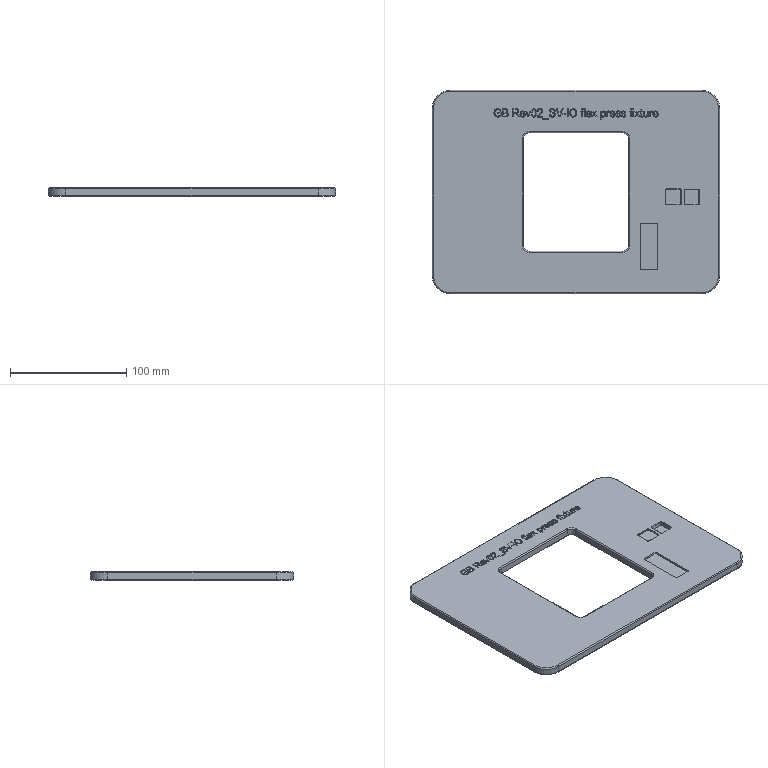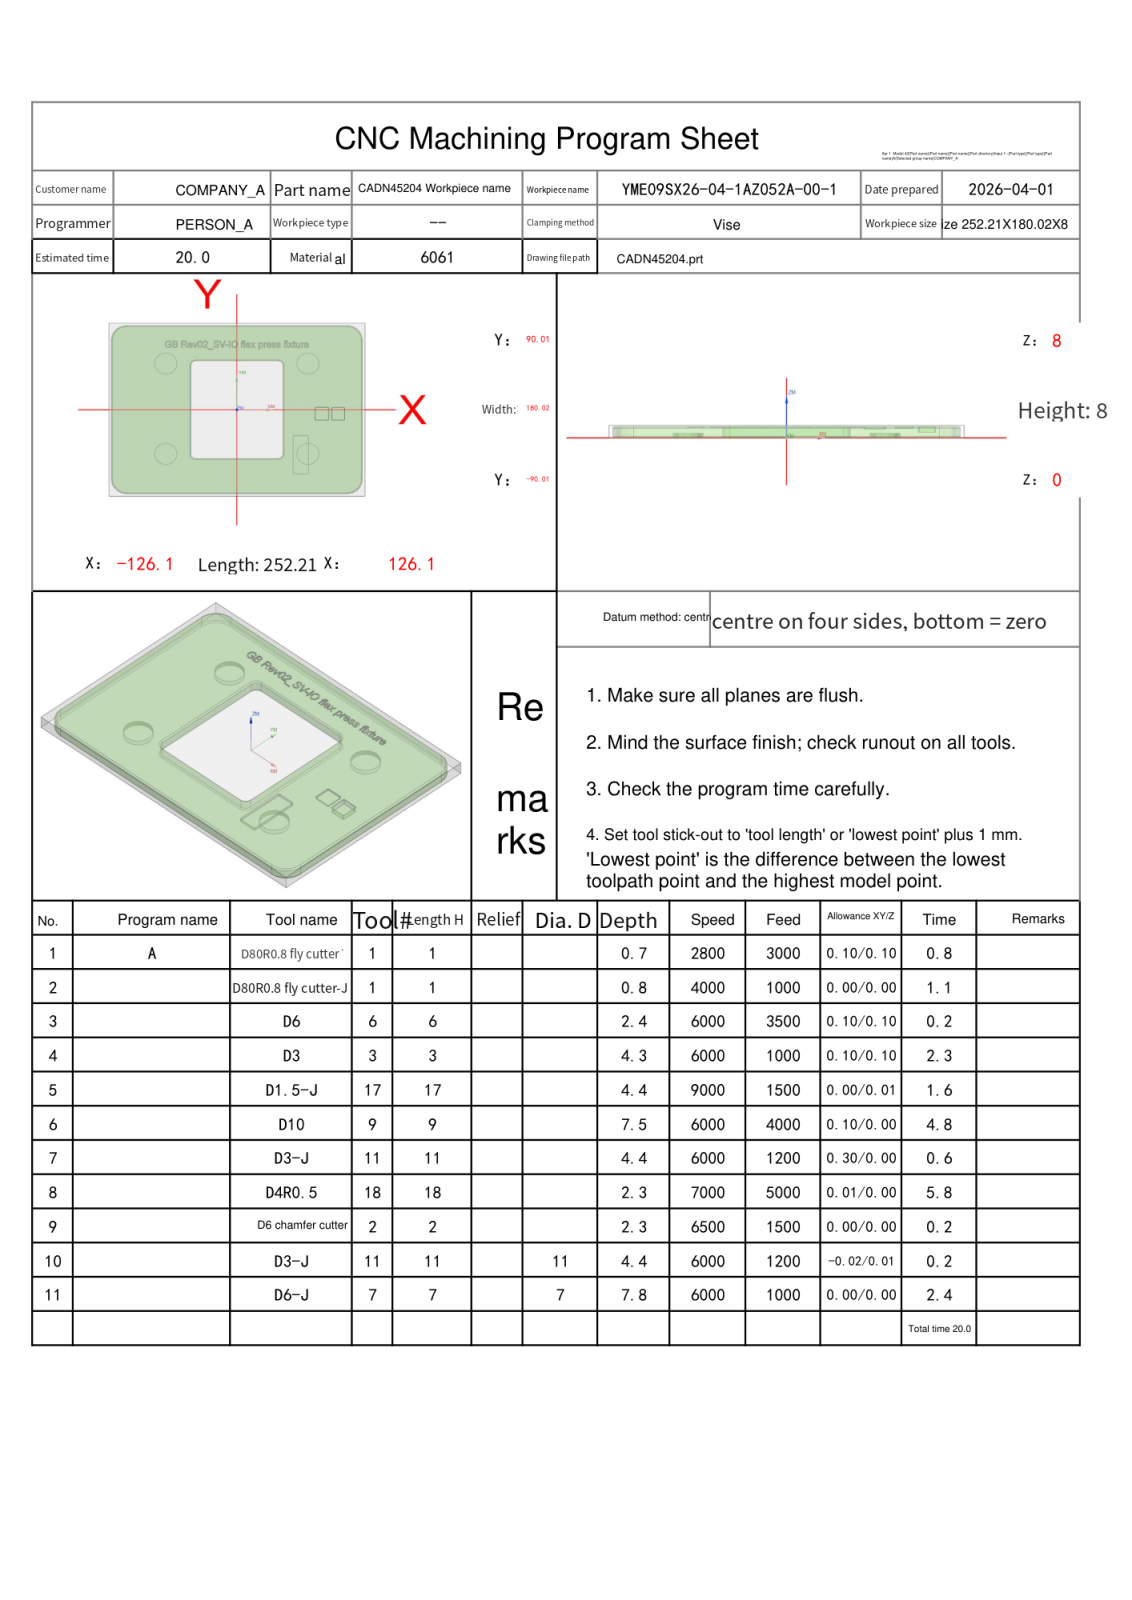NC program | NX | posted by the shop | part box 247.208 x 175.016 x 7.2 mm
Lines 875 to 1934 of 29502:
N5 T17 M06
(D1.5-J  D=1.5 R=0. H=17 ce=0.00 di=0.01)
G00 G90 G54 X56.962 Y-60.982 M03 S9000
G43 H17 Z27.2
M08
Z7.85
G01 X56.953 Y-60.984 Z7.736 F1200.
X56.926 Y-60.99 Z7.634
X56.884 Y-61.002 Z7.542
X56.831 Y-61.019 Z7.461
X56.768 Y-61.043 Z7.389
X56.698 Y-61.073 Z7.327
X56.625 Y-61.11 Z7.274
X56.55 Y-61.155 Z7.229
X56.476 Y-61.208 Z7.191
X56.407 Y-61.27 Z7.161
X56.344 Y-61.342 Z7.138
X56.29 Y-61.423 Z7.121
X56.249 Y-61.515 Z7.109
X56.222 Y-61.617 Z7.102
X56.212 Y-61.732 Z7.1
Y-65.819 F1500.
G03 X56.462 Y-66.069 I.25 J0.0
G01 X60.549
X60.663 Y-66.059 Z7.102
X60.766 Y-66.032 Z7.109
X60.858 Y-65.991 Z7.121
X60.939 Y-65.937 Z7.138
X61.01 Y-65.874 Z7.161
X61.073 Y-65.805 Z7.191
X61.126 Y-65.731 Z7.229
X61.171 Y-65.656 Z7.274
X61.208 Y-65.583 Z7.327
X61.238 Y-65.513 Z7.389
X61.262 Y-65.45 Z7.461
X61.279 Y-65.397 Z7.542
X61.291 Y-65.355 Z7.634
X61.297 Y-65.328 Z7.736
X61.299 Y-65.319 Z7.85
G00 Z10.2
X56.962 Y-60.982
Z7.751
G01 X56.953 Y-60.984 Z7.637 F1200.
X56.926 Y-60.99 Z7.534
X56.884 Y-61.002 Z7.442
X56.831 Y-61.019 Z7.361
X56.768 Y-61.043 Z7.289
X56.698 Y-61.073 Z7.227
X56.625 Y-61.11 Z7.174
X56.55 Y-61.155 Z7.129
X56.476 Y-61.208 Z7.092
X56.407 Y-61.27 Z7.062
X56.344 Y-61.342 Z7.038
X56.29 Y-61.423 Z7.021
X56.249 Y-61.515 Z7.009
X56.222 Y-61.617 Z7.003
X56.212 Y-61.732 Z7.001
Y-65.819 F1500.
G03 X56.462 Y-66.069 I.25 J0.0
G01 X60.549
X60.663 Y-66.059 Z7.003
X60.766 Y-66.032 Z7.009
X60.858 Y-65.991 Z7.021
X60.939 Y-65.937 Z7.038
X61.01 Y-65.874 Z7.062
X61.073 Y-65.805 Z7.092
X61.126 Y-65.731 Z7.129
X61.171 Y-65.656 Z7.174
X61.208 Y-65.583 Z7.227
X61.238 Y-65.513 Z7.289
X61.262 Y-65.45 Z7.361
X61.279 Y-65.397 Z7.442
X61.291 Y-65.355 Z7.534
X61.297 Y-65.328 Z7.637
X61.299 Y-65.319 Z7.751
G00 Z10.1
X56.962 Y-60.982
Z7.651
G01 X56.953 Y-60.984 Z7.537 F1200.
X56.926 Y-60.99 Z7.434
X56.884 Y-61.002 Z7.342
X56.831 Y-61.019 Z7.261
X56.768 Y-61.043 Z7.19
X56.698 Y-61.073 Z7.128
X56.625 Y-61.11 Z7.074
X56.55 Y-61.155 Z7.029
X56.476 Y-61.208 Z6.992
X56.407 Y-61.27 Z6.962
X56.344 Y-61.342 Z6.939
X56.29 Y-61.423 Z6.921
X56.249 Y-61.515 Z6.91
X56.222 Y-61.617 Z6.903
X56.212 Y-61.732 Z6.901
Y-65.819 F1500.
G03 X56.462 Y-66.069 I.25 J0.0
G01 X60.549
X60.663 Y-66.059 Z6.903
X60.766 Y-66.032 Z6.91
X60.858 Y-65.991 Z6.921
X60.939 Y-65.937 Z6.939
X61.01 Y-65.874 Z6.962
X61.073 Y-65.805 Z6.992
X61.126 Y-65.731 Z7.029
X61.171 Y-65.656 Z7.074
X61.208 Y-65.583 Z7.128
X61.238 Y-65.513 Z7.19
X61.262 Y-65.45 Z7.261
X61.279 Y-65.397 Z7.342
X61.291 Y-65.355 Z7.434
X61.297 Y-65.328 Z7.537
X61.299 Y-65.319 Z7.651
G00 Z10.001
X56.962 Y-60.982
Z7.551
G01 X56.953 Y-60.984 Z7.437 F1200.
X56.926 Y-60.99 Z7.334
X56.884 Y-61.002 Z7.243
X56.831 Y-61.019 Z7.161
X56.768 Y-61.043 Z7.09
X56.698 Y-61.073 Z7.028
X56.625 Y-61.11 Z6.975
X56.55 Y-61.155 Z6.93
X56.476 Y-61.208 Z6.892
X56.407 Y-61.27 Z6.862
X56.344 Y-61.342 Z6.839
X56.29 Y-61.423 Z6.822
X56.249 Y-61.515 Z6.81
X56.222 Y-61.617 Z6.803
X56.212 Y-61.732 Z6.801
Y-65.819 F1500.
G03 X56.462 Y-66.069 I.25 J0.0
G01 X60.549
X60.663 Y-66.059 Z6.803
X60.766 Y-66.032 Z6.81
X60.858 Y-65.991 Z6.822
X60.939 Y-65.937 Z6.839
X61.01 Y-65.874 Z6.862
X61.073 Y-65.805 Z6.892
X61.126 Y-65.731 Z6.93
X61.171 Y-65.656 Z6.975
X61.208 Y-65.583 Z7.028
X61.238 Y-65.513 Z7.09
X61.262 Y-65.45 Z7.161
X61.279 Y-65.397 Z7.243
X61.291 Y-65.355 Z7.334
X61.297 Y-65.328 Z7.437
X61.299 Y-65.319 Z7.551
G00 Z9.901
X56.962 Y-60.982
Z7.451
G01 X56.953 Y-60.984 Z7.337 F1200.
X56.926 Y-60.99 Z7.235
X56.884 Y-61.002 Z7.143
X56.831 Y-61.019 Z7.062
X56.768 Y-61.043 Z6.99
X56.698 Y-61.073 Z6.928
X56.625 Y-61.11 Z6.875
X56.55 Y-61.155 Z6.83
X56.476 Y-61.208 Z6.793
X56.407 Y-61.27 Z6.763
X56.344 Y-61.342 Z6.739
X56.29 Y-61.423 Z6.722
X56.249 Y-61.515 Z6.71
X56.222 Y-61.617 Z6.704
X56.212 Y-61.732 Z6.701
Y-65.819 F1500.
G03 X56.462 Y-66.069 I.25 J0.0
G01 X60.549
X60.663 Y-66.059 Z6.704
X60.766 Y-66.032 Z6.71
X60.858 Y-65.991 Z6.722
X60.939 Y-65.937 Z6.739
X61.01 Y-65.874 Z6.763
X61.073 Y-65.805 Z6.793
X61.126 Y-65.731 Z6.83
X61.171 Y-65.656 Z6.875
X61.208 Y-65.583 Z6.928
X61.238 Y-65.513 Z6.99
X61.262 Y-65.45 Z7.062
X61.279 Y-65.397 Z7.143
X61.291 Y-65.355 Z7.235
X61.297 Y-65.328 Z7.337
X61.299 Y-65.319 Z7.451
G00 Z9.801
X56.962 Y-60.982
Z7.352
G01 X56.953 Y-60.984 Z7.238 F1200.
X56.926 Y-60.99 Z7.135
X56.884 Y-61.002 Z7.043
X56.831 Y-61.019 Z6.962
X56.768 Y-61.043 Z6.891
X56.698 Y-61.073 Z6.829
X56.625 Y-61.11 Z6.775
X56.55 Y-61.155 Z6.73
X56.476 Y-61.208 Z6.693
X56.407 Y-61.27 Z6.663
X56.344 Y-61.342 Z6.639
X56.29 Y-61.423 Z6.622
X56.249 Y-61.515 Z6.61
X56.222 Y-61.617 Z6.604
X56.212 Y-61.732 Z6.602
Y-65.819 F1500.
G03 X56.462 Y-66.069 I.25 J0.0
G01 X60.549
X60.663 Y-66.059 Z6.604
X60.766 Y-66.032 Z6.61
X60.858 Y-65.991 Z6.622
X60.939 Y-65.937 Z6.639
X61.01 Y-65.874 Z6.663
X61.073 Y-65.805 Z6.693
X61.126 Y-65.731 Z6.73
X61.171 Y-65.656 Z6.775
X61.208 Y-65.583 Z6.829
X61.238 Y-65.513 Z6.891
X61.262 Y-65.45 Z6.962
X61.279 Y-65.397 Z7.043
X61.291 Y-65.355 Z7.135
X61.297 Y-65.328 Z7.238
X61.299 Y-65.319 Z7.352
G00 Z9.701
X56.962 Y-60.982
Z7.252
G01 X56.953 Y-60.984 Z7.138 F1200.
X56.926 Y-60.99 Z7.035
X56.884 Y-61.002 Z6.944
X56.831 Y-61.019 Z6.862
X56.768 Y-61.043 Z6.791
X56.698 Y-61.073 Z6.729
X56.625 Y-61.11 Z6.676
X56.55 Y-61.155 Z6.631
X56.476 Y-61.208 Z6.593
X56.407 Y-61.27 Z6.563
X56.344 Y-61.342 Z6.54
X56.29 Y-61.423 Z6.522
X56.249 Y-61.515 Z6.511
X56.222 Y-61.617 Z6.504
X56.212 Y-61.732 Z6.502
Y-65.819 F1500.
G03 X56.462 Y-66.069 I.25 J0.0
G01 X60.549
X60.663 Y-66.059 Z6.504
X60.766 Y-66.032 Z6.511
X60.858 Y-65.991 Z6.522
X60.939 Y-65.937 Z6.54
X61.01 Y-65.874 Z6.563
X61.073 Y-65.805 Z6.593
X61.126 Y-65.731 Z6.631
X61.171 Y-65.656 Z6.676
X61.208 Y-65.583 Z6.729
X61.238 Y-65.513 Z6.791
X61.262 Y-65.45 Z6.862
X61.279 Y-65.397 Z6.944
X61.291 Y-65.355 Z7.035
X61.297 Y-65.328 Z7.138
X61.299 Y-65.319 Z7.252
G00 Z9.602
X56.962 Y-60.982
Z7.152
G01 X56.953 Y-60.984 Z7.038 F1200.
X56.926 Y-60.99 Z6.936
X56.884 Y-61.002 Z6.844
X56.831 Y-61.019 Z6.763
X56.768 Y-61.043 Z6.691
X56.698 Y-61.073 Z6.629
X56.625 Y-61.11 Z6.576
X56.55 Y-61.155 Z6.531
X56.476 Y-61.208 Z6.494
X56.407 Y-61.27 Z6.463
X56.344 Y-61.342 Z6.44
X56.29 Y-61.423 Z6.423
X56.249 Y-61.515 Z6.411
X56.222 Y-61.617 Z6.404
X56.212 Y-61.732 Z6.402
Y-65.819 F1500.
G03 X56.462 Y-66.069 I.25 J0.0
G01 X60.549
X60.663 Y-66.059 Z6.404
X60.766 Y-66.032 Z6.411
X60.858 Y-65.991 Z6.423
X60.939 Y-65.937 Z6.44
X61.01 Y-65.874 Z6.463
X61.073 Y-65.805 Z6.494
X61.126 Y-65.731 Z6.531
X61.171 Y-65.656 Z6.576
X61.208 Y-65.583 Z6.629
X61.238 Y-65.513 Z6.691
X61.262 Y-65.45 Z6.763
X61.279 Y-65.397 Z6.844
X61.291 Y-65.355 Z6.936
X61.297 Y-65.328 Z7.038
X61.299 Y-65.319 Z7.152
G00 Z9.502
X56.962 Y-60.982
Z7.053
G01 X56.953 Y-60.984 Z6.939 F1200.
X56.926 Y-60.99 Z6.836
X56.884 Y-61.002 Z6.744
X56.831 Y-61.019 Z6.663
X56.768 Y-61.043 Z6.592
X56.698 Y-61.073 Z6.529
X56.625 Y-61.11 Z6.476
X56.55 Y-61.155 Z6.431
X56.476 Y-61.208 Z6.394
X56.407 Y-61.27 Z6.364
X56.344 Y-61.342 Z6.34
X56.29 Y-61.423 Z6.323
X56.249 Y-61.515 Z6.311
X56.222 Y-61.617 Z6.305
X56.212 Y-61.732 Z6.303
Y-65.819 F1500.
G03 X56.462 Y-66.069 I.25 J0.0
G01 X60.549
X60.663 Y-66.059 Z6.305
X60.766 Y-66.032 Z6.311
X60.858 Y-65.991 Z6.323
X60.939 Y-65.937 Z6.34
X61.01 Y-65.874 Z6.364
X61.073 Y-65.805 Z6.394
X61.126 Y-65.731 Z6.431
X61.171 Y-65.656 Z6.476
X61.208 Y-65.583 Z6.529
X61.238 Y-65.513 Z6.592
X61.262 Y-65.45 Z6.663
X61.279 Y-65.397 Z6.744
X61.291 Y-65.355 Z6.836
X61.297 Y-65.328 Z6.939
X61.299 Y-65.319 Z7.053
G00 Z9.402
X56.962 Y-60.982
Z6.953
G01 X56.953 Y-60.984 Z6.839 F1200.
X56.926 Y-60.99 Z6.736
X56.884 Y-61.002 Z6.645
X56.831 Y-61.019 Z6.563
X56.768 Y-61.043 Z6.492
X56.698 Y-61.073 Z6.43
X56.625 Y-61.11 Z6.376
X56.55 Y-61.155 Z6.331
X56.476 Y-61.208 Z6.294
X56.407 Y-61.27 Z6.264
X56.344 Y-61.342 Z6.241
X56.29 Y-61.423 Z6.223
X56.249 Y-61.515 Z6.212
X56.222 Y-61.617 Z6.205
X56.212 Y-61.732 Z6.203
Y-65.819 F1500.
G03 X56.462 Y-66.069 I.25 J0.0
G01 X60.549
X60.663 Y-66.059 Z6.205
X60.766 Y-66.032 Z6.212
X60.858 Y-65.991 Z6.223
X60.939 Y-65.937 Z6.241
X61.01 Y-65.874 Z6.264
X61.073 Y-65.805 Z6.294
X61.126 Y-65.731 Z6.331
X61.171 Y-65.656 Z6.376
X61.208 Y-65.583 Z6.43
X61.238 Y-65.513 Z6.492
X61.262 Y-65.45 Z6.563
X61.279 Y-65.397 Z6.645
X61.291 Y-65.355 Z6.736
X61.297 Y-65.328 Z6.839
X61.299 Y-65.319 Z6.953
G00 Z9.303
X56.962 Y-60.982
Z6.853
G01 X56.953 Y-60.984 Z6.739 F1200.
X56.926 Y-60.99 Z6.637
X56.884 Y-61.002 Z6.545
X56.831 Y-61.019 Z6.464
X56.768 Y-61.043 Z6.392
X56.698 Y-61.073 Z6.33
X56.625 Y-61.11 Z6.277
X56.55 Y-61.155 Z6.232
X56.476 Y-61.208 Z6.194
X56.407 Y-61.27 Z6.164
X56.344 Y-61.342 Z6.141
X56.29 Y-61.423 Z6.124
X56.249 Y-61.515 Z6.112
X56.222 Y-61.617 Z6.105
X56.212 Y-61.732 Z6.103
Y-65.819 F1500.
G03 X56.462 Y-66.069 I.25 J0.0
G01 X60.549
X60.663 Y-66.059 Z6.105
X60.766 Y-66.032 Z6.112
X60.858 Y-65.991 Z6.124
X60.939 Y-65.937 Z6.141
X61.01 Y-65.874 Z6.164
X61.073 Y-65.805 Z6.194
X61.126 Y-65.731 Z6.232
X61.171 Y-65.656 Z6.277
X61.208 Y-65.583 Z6.33
X61.238 Y-65.513 Z6.392
X61.262 Y-65.45 Z6.464
X61.279 Y-65.397 Z6.545
X61.291 Y-65.355 Z6.637
X61.297 Y-65.328 Z6.739
X61.299 Y-65.319 Z6.853
G00 Z9.203
X56.962 Y-60.982
Z6.754
G01 X56.953 Y-60.984 Z6.639 F1200.
X56.926 Y-60.99 Z6.537
X56.884 Y-61.002 Z6.445
X56.831 Y-61.019 Z6.364
X56.768 Y-61.043 Z6.292
X56.698 Y-61.073 Z6.23
X56.625 Y-61.11 Z6.177
X56.55 Y-61.155 Z6.132
X56.476 Y-61.208 Z6.095
X56.407 Y-61.27 Z6.065
X56.344 Y-61.342 Z6.041
X56.29 Y-61.423 Z6.024
X56.249 Y-61.515 Z6.012
X56.222 Y-61.617 Z6.006
X56.212 Y-61.732 Z6.004
Y-65.819 F1500.
G03 X56.462 Y-66.069 I.25 J0.0
G01 X60.549
X60.663 Y-66.059 Z6.006
X60.766 Y-66.032 Z6.012
X60.858 Y-65.991 Z6.024
X60.939 Y-65.937 Z6.041
X61.01 Y-65.874 Z6.065
X61.073 Y-65.805 Z6.095
X61.126 Y-65.731 Z6.132
X61.171 Y-65.656 Z6.177
X61.208 Y-65.583 Z6.23
X61.238 Y-65.513 Z6.292
X61.262 Y-65.45 Z6.364
X61.279 Y-65.397 Z6.445
X61.291 Y-65.355 Z6.537
X61.297 Y-65.328 Z6.639
X61.299 Y-65.319 Z6.754
G00 Z9.103
X56.962 Y-60.982
Z6.654
G01 X56.953 Y-60.984 Z6.54 F1200.
X56.926 Y-60.99 Z6.437
X56.884 Y-61.002 Z6.345
X56.831 Y-61.019 Z6.264
X56.768 Y-61.043 Z6.193
X56.698 Y-61.073 Z6.131
X56.625 Y-61.11 Z6.077
X56.55 Y-61.155 Z6.032
X56.476 Y-61.208 Z5.995
X56.407 Y-61.27 Z5.965
X56.344 Y-61.342 Z5.942
X56.29 Y-61.423 Z5.924
X56.249 Y-61.515 Z5.913
X56.222 Y-61.617 Z5.906
X56.212 Y-61.732 Z5.904
Y-65.819 F1500.
G03 X56.462 Y-66.069 I.25 J0.0
G01 X60.549
X60.663 Y-66.059 Z5.906
X60.766 Y-66.032 Z5.913
X60.858 Y-65.991 Z5.924
X60.939 Y-65.937 Z5.942
X61.01 Y-65.874 Z5.965
X61.073 Y-65.805 Z5.995
X61.126 Y-65.731 Z6.032
X61.171 Y-65.656 Z6.077
X61.208 Y-65.583 Z6.131
X61.238 Y-65.513 Z6.193
X61.262 Y-65.45 Z6.264
X61.279 Y-65.397 Z6.345
X61.291 Y-65.355 Z6.437
X61.297 Y-65.328 Z6.54
X61.299 Y-65.319 Z6.654
G00 Z9.004
X56.962 Y-60.982
Z6.554
G01 X56.953 Y-60.984 Z6.44 F1200.
X56.926 Y-60.99 Z6.337
X56.884 Y-61.002 Z6.246
X56.831 Y-61.019 Z6.164
X56.768 Y-61.043 Z6.093
X56.698 Y-61.073 Z6.031
X56.625 Y-61.11 Z5.978
X56.55 Y-61.155 Z5.933
X56.476 Y-61.208 Z5.895
X56.407 Y-61.27 Z5.865
X56.344 Y-61.342 Z5.842
X56.29 Y-61.423 Z5.825
X56.249 Y-61.515 Z5.813
X56.222 Y-61.617 Z5.806
X56.212 Y-61.732 Z5.804
Y-65.819 F1500.
G03 X56.462 Y-66.069 I.25 J0.0
G01 X60.549
X60.663 Y-66.059 Z5.806
X60.766 Y-66.032 Z5.813
X60.858 Y-65.991 Z5.825
X60.939 Y-65.937 Z5.842
X61.01 Y-65.874 Z5.865
X61.073 Y-65.805 Z5.895
X61.126 Y-65.731 Z5.933
X61.171 Y-65.656 Z5.978
X61.208 Y-65.583 Z6.031
X61.238 Y-65.513 Z6.093
X61.262 Y-65.45 Z6.164
X61.279 Y-65.397 Z6.246
X61.291 Y-65.355 Z6.337
X61.297 Y-65.328 Z6.44
X61.299 Y-65.319 Z6.554
G00 Z8.904
X56.962 Y-60.982
Z6.454
G01 X56.953 Y-60.984 Z6.34 F1200.
X56.926 Y-60.99 Z6.238
X56.884 Y-61.002 Z6.146
X56.831 Y-61.019 Z6.065
X56.768 Y-61.043 Z5.993
X56.698 Y-61.073 Z5.931
X56.625 Y-61.11 Z5.878
X56.55 Y-61.155 Z5.833
X56.476 Y-61.208 Z5.796
X56.407 Y-61.27 Z5.766
X56.344 Y-61.342 Z5.742
X56.29 Y-61.423 Z5.725
X56.249 Y-61.515 Z5.713
X56.222 Y-61.617 Z5.707
X56.212 Y-61.732 Z5.704
Y-65.819 F1500.
G03 X56.462 Y-66.069 I.25 J0.0
G01 X60.549
X60.663 Y-66.059 Z5.707
X60.766 Y-66.032 Z5.713
X60.858 Y-65.991 Z5.725
X60.939 Y-65.937 Z5.742
X61.01 Y-65.874 Z5.766
X61.073 Y-65.805 Z5.796
X61.126 Y-65.731 Z5.833
X61.171 Y-65.656 Z5.878
X61.208 Y-65.583 Z5.931
X61.238 Y-65.513 Z5.993
X61.262 Y-65.45 Z6.065
X61.279 Y-65.397 Z6.146
X61.291 Y-65.355 Z6.238
X61.297 Y-65.328 Z6.34
X61.299 Y-65.319 Z6.454
G00 Z8.804
X56.962 Y-60.982
Z6.355
G01 X56.953 Y-60.984 Z6.241 F1200.
X56.926 Y-60.99 Z6.138
X56.884 Y-61.002 Z6.046
X56.831 Y-61.019 Z5.965
X56.768 Y-61.043 Z5.894
X56.698 Y-61.073 Z5.832
X56.625 Y-61.11 Z5.778
X56.55 Y-61.155 Z5.733
X56.476 Y-61.208 Z5.696
X56.407 Y-61.27 Z5.666
X56.344 Y-61.342 Z5.642
X56.29 Y-61.423 Z5.625
X56.249 Y-61.515 Z5.613
X56.222 Y-61.617 Z5.607
X56.212 Y-61.732 Z5.605
Y-65.819 F1500.
G03 X56.462 Y-66.069 I.25 J0.0
G01 X60.549
X60.663 Y-66.059 Z5.607
X60.766 Y-66.032 Z5.613
X60.858 Y-65.991 Z5.625
X60.939 Y-65.937 Z5.642
X61.01 Y-65.874 Z5.666
X61.073 Y-65.805 Z5.696
X61.126 Y-65.731 Z5.733
X61.171 Y-65.656 Z5.778
X61.208 Y-65.583 Z5.832
X61.238 Y-65.513 Z5.894
X61.262 Y-65.45 Z5.965
X61.279 Y-65.397 Z6.046
X61.291 Y-65.355 Z6.138
X61.297 Y-65.328 Z6.241
X61.299 Y-65.319 Z6.355
G00 Z8.704
X56.962 Y-60.982
Z6.255
G01 X56.953 Y-60.984 Z6.141 F1200.
X56.926 Y-60.99 Z6.038
X56.884 Y-61.002 Z5.947
X56.831 Y-61.019 Z5.865
X56.768 Y-61.043 Z5.794
X56.698 Y-61.073 Z5.732
X56.625 Y-61.11 Z5.679
X56.55 Y-61.155 Z5.633
X56.476 Y-61.208 Z5.596
X56.407 Y-61.27 Z5.566
X56.344 Y-61.342 Z5.543
X56.29 Y-61.423 Z5.525
X56.249 Y-61.515 Z5.514
X56.222 Y-61.617 Z5.507
X56.212 Y-61.732 Z5.505
Y-65.819 F1500.
G03 X56.462 Y-66.069 I.25 J0.0
G01 X60.549
X60.663 Y-66.059 Z5.507
X60.766 Y-66.032 Z5.514
X60.858 Y-65.991 Z5.525
X60.939 Y-65.937 Z5.543
X61.01 Y-65.874 Z5.566
X61.073 Y-65.805 Z5.596
X61.126 Y-65.731 Z5.633
X61.171 Y-65.656 Z5.679
X61.208 Y-65.583 Z5.732
X61.238 Y-65.513 Z5.794
X61.262 Y-65.45 Z5.865
X61.279 Y-65.397 Z5.947
X61.291 Y-65.355 Z6.038
X61.297 Y-65.328 Z6.141
X61.299 Y-65.319 Z6.255
G00 Z10.2
X64.625
Z7.85
G01 X64.627 Y-65.328 Z7.736 F1200.
X64.634 Y-65.355 Z7.634
X64.645 Y-65.397 Z7.542
X64.663 Y-65.45 Z7.461
X64.686 Y-65.513 Z7.389
X64.716 Y-65.583 Z7.327
X64.753 Y-65.656 Z7.274
X64.798 Y-65.731 Z7.229
X64.852 Y-65.805 Z7.191
X64.914 Y-65.874 Z7.161
X64.985 Y-65.937 Z7.138
X65.067 Y-65.991 Z7.121
X65.158 Y-66.032 Z7.109
X65.261 Y-66.059 Z7.102
X65.375 Y-66.069 Z7.1
X69.462 F1500.
G03 X69.712 Y-65.819 I0.0 J.25
G01 Y-61.732
X69.703 Y-61.617 Z7.102
X69.676 Y-61.515 Z7.109
X69.634 Y-61.423 Z7.121
X69.581 Y-61.342 Z7.138
X69.518 Y-61.27 Z7.161
X69.448 Y-61.208 Z7.191
X69.375 Y-61.155 Z7.229
X69.3 Y-61.11 Z7.274
X69.226 Y-61.073 Z7.327
X69.157 Y-61.043 Z7.389
X69.094 Y-61.019 Z7.461
X69.04 Y-61.002 Z7.542
X68.999 Y-60.99 Z7.634
X68.972 Y-60.984 Z7.736
X68.962 Y-60.982 Z7.85
G00 Z10.2
X64.625 Y-65.319
Z7.751
G01 X64.627 Y-65.328 Z7.637 F1200.
X64.634 Y-65.355 Z7.534
X64.645 Y-65.397 Z7.442
X64.663 Y-65.45 Z7.361
X64.686 Y-65.513 Z7.289
X64.716 Y-65.583 Z7.227
X64.753 Y-65.656 Z7.174
X64.798 Y-65.731 Z7.129
X64.852 Y-65.805 Z7.092
X64.914 Y-65.874 Z7.062
X64.985 Y-65.937 Z7.038
X65.067 Y-65.991 Z7.021
X65.158 Y-66.032 Z7.009
X65.261 Y-66.059 Z7.003
X65.375 Y-66.069 Z7.001
X69.462 F1500.
G03 X69.712 Y-65.819 I0.0 J.25
G01 Y-61.732
X69.703 Y-61.617 Z7.003
X69.676 Y-61.515 Z7.009
X69.634 Y-61.423 Z7.021
X69.581 Y-61.342 Z7.038
X69.518 Y-61.27 Z7.062
X69.448 Y-61.208 Z7.092
X69.375 Y-61.155 Z7.129
X69.3 Y-61.11 Z7.174
X69.226 Y-61.073 Z7.227
X69.157 Y-61.043 Z7.289
X69.094 Y-61.019 Z7.361
X69.04 Y-61.002 Z7.442
X68.999 Y-60.99 Z7.534
X68.972 Y-60.984 Z7.637
X68.962 Y-60.982 Z7.751
G00 Z10.1
X64.625 Y-65.319
Z7.651
G01 X64.627 Y-65.328 Z7.537 F1200.
X64.634 Y-65.355 Z7.434
X64.645 Y-65.397 Z7.342
X64.663 Y-65.45 Z7.261
X64.686 Y-65.513 Z7.19
X64.716 Y-65.583 Z7.128
X64.753 Y-65.656 Z7.074
X64.798 Y-65.731 Z7.029
X64.852 Y-65.805 Z6.992
X64.914 Y-65.874 Z6.962
X64.985 Y-65.937 Z6.939
X65.067 Y-65.991 Z6.921
X65.158 Y-66.032 Z6.91
X65.261 Y-66.059 Z6.903
X65.375 Y-66.069 Z6.901
X69.462 F1500.
G03 X69.712 Y-65.819 I0.0 J.25
G01 Y-61.732
X69.703 Y-61.617 Z6.903
X69.676 Y-61.515 Z6.91
X69.634 Y-61.423 Z6.921
X69.581 Y-61.342 Z6.939
X69.518 Y-61.27 Z6.962
X69.448 Y-61.208 Z6.992
X69.375 Y-61.155 Z7.029
X69.3 Y-61.11 Z7.074
X69.226 Y-61.073 Z7.128
X69.157 Y-61.043 Z7.19
X69.094 Y-61.019 Z7.261
X69.04 Y-61.002 Z7.342
X68.999 Y-60.99 Z7.434
X68.972 Y-60.984 Z7.537
X68.962 Y-60.982 Z7.651
G00 Z10.001
X64.625 Y-65.319
Z7.551
G01 X64.627 Y-65.328 Z7.437 F1200.
X64.634 Y-65.355 Z7.334
X64.645 Y-65.397 Z7.243
X64.663 Y-65.45 Z7.161
X64.686 Y-65.513 Z7.09
X64.716 Y-65.583 Z7.028
X64.753 Y-65.656 Z6.975
X64.798 Y-65.731 Z6.93
X64.852 Y-65.805 Z6.892
X64.914 Y-65.874 Z6.862
X64.985 Y-65.937 Z6.839
X65.067 Y-65.991 Z6.822
X65.158 Y-66.032 Z6.81
X65.261 Y-66.059 Z6.803
X65.375 Y-66.069 Z6.801
X69.462 F1500.
G03 X69.712 Y-65.819 I0.0 J.25
G01 Y-61.732
X69.703 Y-61.617 Z6.803
X69.676 Y-61.515 Z6.81
X69.634 Y-61.423 Z6.822
X69.581 Y-61.342 Z6.839
X69.518 Y-61.27 Z6.862
X69.448 Y-61.208 Z6.892
X69.375 Y-61.155 Z6.93
X69.3 Y-61.11 Z6.975
X69.226 Y-61.073 Z7.028
X69.157 Y-61.043 Z7.09
X69.094 Y-61.019 Z7.161
X69.04 Y-61.002 Z7.243
X68.999 Y-60.99 Z7.334
X68.972 Y-60.984 Z7.437
X68.962 Y-60.982 Z7.551
G00 Z9.901
X64.625 Y-65.319
Z7.451
G01 X64.627 Y-65.328 Z7.337 F1200.
X64.634 Y-65.355 Z7.235
X64.645 Y-65.397 Z7.143
X64.663 Y-65.45 Z7.062
X64.686 Y-65.513 Z6.99
X64.716 Y-65.583 Z6.928
X64.753 Y-65.656 Z6.875
X64.798 Y-65.731 Z6.83
X64.852 Y-65.805 Z6.793
X64.914 Y-65.874 Z6.763
X64.985 Y-65.937 Z6.739
X65.067 Y-65.991 Z6.722
X65.158 Y-66.032 Z6.71
X65.261 Y-66.059 Z6.704
X65.375 Y-66.069 Z6.701
X69.462 F1500.
G03 X69.712 Y-65.819 I0.0 J.25
G01 Y-61.732
X69.703 Y-61.617 Z6.704
X69.676 Y-61.515 Z6.71
X69.634 Y-61.423 Z6.722
X69.581 Y-61.342 Z6.739
X69.518 Y-61.27 Z6.763
X69.448 Y-61.208 Z6.793
X69.375 Y-61.155 Z6.83
X69.3 Y-61.11 Z6.875
X69.226 Y-61.073 Z6.928
X69.157 Y-61.043 Z6.99
X69.094 Y-61.019 Z7.062
X69.04 Y-61.002 Z7.143
X68.999 Y-60.99 Z7.235
X68.972 Y-60.984 Z7.337
X68.962 Y-60.982 Z7.451
G00 Z9.801
X64.625 Y-65.319
Z7.352
G01 X64.627 Y-65.328 Z7.238 F1200.
X64.634 Y-65.355 Z7.135
X64.645 Y-65.397 Z7.043
X64.663 Y-65.45 Z6.962
X64.686 Y-65.513 Z6.891
X64.716 Y-65.583 Z6.829
X64.753 Y-65.656 Z6.775
X64.798 Y-65.731 Z6.73
X64.852 Y-65.805 Z6.693
X64.914 Y-65.874 Z6.663
X64.985 Y-65.937 Z6.639
X65.067 Y-65.991 Z6.622
X65.158 Y-66.032 Z6.61
X65.261 Y-66.059 Z6.604
X65.375 Y-66.069 Z6.602
X69.462 F1500.
G03 X69.712 Y-65.819 I0.0 J.25
G01 Y-61.732
X69.703 Y-61.617 Z6.604
X69.676 Y-61.515 Z6.61
X69.634 Y-61.423 Z6.622
X69.581 Y-61.342 Z6.639
X69.518 Y-61.27 Z6.663
X69.448 Y-61.208 Z6.693
X69.375 Y-61.155 Z6.73
X69.3 Y-61.11 Z6.775
X69.226 Y-61.073 Z6.829
X69.157 Y-61.043 Z6.891
X69.094 Y-61.019 Z6.962
X69.04 Y-61.002 Z7.043
X68.999 Y-60.99 Z7.135
X68.972 Y-60.984 Z7.238
X68.962 Y-60.982 Z7.352
G00 Z9.701
X64.625 Y-65.319
Z7.252
G01 X64.627 Y-65.328 Z7.138 F1200.
X64.634 Y-65.355 Z7.035
X64.645 Y-65.397 Z6.944
X64.663 Y-65.45 Z6.862
X64.686 Y-65.513 Z6.791
X64.716 Y-65.583 Z6.729
X64.753 Y-65.656 Z6.676
X64.798 Y-65.731 Z6.631
X64.852 Y-65.805 Z6.593
X64.914 Y-65.874 Z6.563
X64.985 Y-65.937 Z6.54
X65.067 Y-65.991 Z6.522
X65.158 Y-66.032 Z6.511
X65.261 Y-66.059 Z6.504
X65.375 Y-66.069 Z6.502
X69.462 F1500.
G03 X69.712 Y-65.819 I0.0 J.25
G01 Y-61.732
X69.703 Y-61.617 Z6.504
X69.676 Y-61.515 Z6.511
X69.634 Y-61.423 Z6.522
X69.581 Y-61.342 Z6.54
X69.518 Y-61.27 Z6.563
X69.448 Y-61.208 Z6.593
X69.375 Y-61.155 Z6.631
X69.3 Y-61.11 Z6.676
X69.226 Y-61.073 Z6.729
X69.157 Y-61.043 Z6.791
X69.094 Y-61.019 Z6.862
X69.04 Y-61.002 Z6.944
X68.999 Y-60.99 Z7.035
X68.972 Y-60.984 Z7.138
X68.962 Y-60.982 Z7.252
G00 Z9.602
X64.625 Y-65.319
Z7.152
G01 X64.627 Y-65.328 Z7.038 F1200.
X64.634 Y-65.355 Z6.936
X64.645 Y-65.397 Z6.844
X64.663 Y-65.45 Z6.763
X64.686 Y-65.513 Z6.691
X64.716 Y-65.583 Z6.629
X64.753 Y-65.656 Z6.576
X64.798 Y-65.731 Z6.531
X64.852 Y-65.805 Z6.494
X64.914 Y-65.874 Z6.463
X64.985 Y-65.937 Z6.44
X65.067 Y-65.991 Z6.423
X65.158 Y-66.032 Z6.411
X65.261 Y-66.059 Z6.404
X65.375 Y-66.069 Z6.402
X69.462 F1500.
G03 X69.712 Y-65.819 I0.0 J.25
G01 Y-61.732
X69.703 Y-61.617 Z6.404
X69.676 Y-61.515 Z6.411
X69.634 Y-61.423 Z6.423
X69.581 Y-61.342 Z6.44
X69.518 Y-61.27 Z6.463
X69.448 Y-61.208 Z6.494
X69.375 Y-61.155 Z6.531
X69.3 Y-61.11 Z6.576
X69.226 Y-61.073 Z6.629
X69.157 Y-61.043 Z6.691
X69.094 Y-61.019 Z6.763
X69.04 Y-61.002 Z6.844
X68.999 Y-60.99 Z6.936
X68.972 Y-60.984 Z7.038
X68.962 Y-60.982 Z7.152
G00 Z9.502
X64.625 Y-65.319
Z7.053
G01 X64.627 Y-65.328 Z6.939 F1200.
X64.634 Y-65.355 Z6.836
X64.645 Y-65.397 Z6.744
X64.663 Y-65.45 Z6.663
X64.686 Y-65.513 Z6.592
X64.716 Y-65.583 Z6.529
X64.753 Y-65.656 Z6.476
X64.798 Y-65.731 Z6.431
X64.852 Y-65.805 Z6.394
X64.914 Y-65.874 Z6.364
X64.985 Y-65.937 Z6.34
X65.067 Y-65.991 Z6.323
X65.158 Y-66.032 Z6.311
X65.261 Y-66.059 Z6.305
X65.375 Y-66.069 Z6.303
X69.462 F1500.
G03 X69.712 Y-65.819 I0.0 J.25
G01 Y-61.732
X69.703 Y-61.617 Z6.305
X69.676 Y-61.515 Z6.311
X69.634 Y-61.423 Z6.323
X69.581 Y-61.342 Z6.34
X69.518 Y-61.27 Z6.364
X69.448 Y-61.208 Z6.394
X69.375 Y-61.155 Z6.431
X69.3 Y-61.11 Z6.476
X69.226 Y-61.073 Z6.529
X69.157 Y-61.043 Z6.592
X69.094 Y-61.019 Z6.663
X69.04 Y-61.002 Z6.744
X68.999 Y-60.99 Z6.836
X68.972 Y-60.984 Z6.939
X68.962 Y-60.982 Z7.053
G00 Z9.402
X64.625 Y-65.319
Z6.953
G01 X64.627 Y-65.328 Z6.839 F1200.
X64.634 Y-65.355 Z6.736
X64.645 Y-65.397 Z6.645
X64.663 Y-65.45 Z6.563
X64.686 Y-65.513 Z6.492
X64.716 Y-65.583 Z6.43
X64.753 Y-65.656 Z6.376
X64.798 Y-65.731 Z6.331
X64.852 Y-65.805 Z6.294
X64.914 Y-65.874 Z6.264
X64.985 Y-65.937 Z6.241
X65.067 Y-65.991 Z6.223
X65.158 Y-66.032 Z6.212
X65.261 Y-66.059 Z6.205
X65.375 Y-66.069 Z6.203
X69.462 F1500.
G03 X69.712 Y-65.819 I0.0 J.25
G01 Y-61.732
X69.703 Y-61.617 Z6.205
X69.676 Y-61.515 Z6.212
X69.634 Y-61.423 Z6.223
X69.581 Y-61.342 Z6.241
X69.518 Y-61.27 Z6.264
X69.448 Y-61.208 Z6.294
X69.375 Y-61.155 Z6.331
X69.3 Y-61.11 Z6.376
X69.226 Y-61.073 Z6.43
X69.157 Y-61.043 Z6.492
X69.094 Y-61.019 Z6.563
X69.04 Y-61.002 Z6.645
X68.999 Y-60.99 Z6.736
X68.972 Y-60.984 Z6.839
X68.962 Y-60.982 Z6.953
G00 Z9.303
X64.625 Y-65.319
Z6.853
G01 X64.627 Y-65.328 Z6.739 F1200.
X64.634 Y-65.355 Z6.637
X64.645 Y-65.397 Z6.545
X64.663 Y-65.45 Z6.464
X64.686 Y-65.513 Z6.392
X64.716 Y-65.583 Z6.33
X64.753 Y-65.656 Z6.277
X64.798 Y-65.731 Z6.232
X64.852 Y-65.805 Z6.194
X64.914 Y-65.874 Z6.164
X64.985 Y-65.937 Z6.141
X65.067 Y-65.991 Z6.124
X65.158 Y-66.032 Z6.112
X65.261 Y-66.059 Z6.105
X65.375 Y-66.069 Z6.103
X69.462 F1500.
G03 X69.712 Y-65.819 I0.0 J.25
G01 Y-61.732
X69.703 Y-61.617 Z6.105
X69.676 Y-61.515 Z6.112
X69.634 Y-61.423 Z6.124
X69.581 Y-61.342 Z6.141
X69.518 Y-61.27 Z6.164
X69.448 Y-61.208 Z6.194
X69.375 Y-61.155 Z6.232
X69.3 Y-61.11 Z6.277
X69.226 Y-61.073 Z6.33
X69.157 Y-61.043 Z6.392
X69.094 Y-61.019 Z6.464
X69.04 Y-61.002 Z6.545
X68.999 Y-60.99 Z6.637
X68.972 Y-60.984 Z6.739
X68.962 Y-60.982 Z6.853
G00 Z9.203
X64.625 Y-65.319
Z6.754
G01 X64.627 Y-65.328 Z6.639 F1200.
X64.634 Y-65.355 Z6.537
X64.645 Y-65.397 Z6.445
X64.663 Y-65.45 Z6.364
X64.686 Y-65.513 Z6.292
X64.716 Y-65.583 Z6.23
X64.753 Y-65.656 Z6.177
X64.798 Y-65.731 Z6.132
X64.852 Y-65.805 Z6.095
X64.914 Y-65.874 Z6.065
X64.985 Y-65.937 Z6.041
X65.067 Y-65.991 Z6.024
X65.158 Y-66.032 Z6.012
X65.261 Y-66.059 Z6.006
X65.375 Y-66.069 Z6.004
X69.462 F1500.
G03 X69.712 Y-65.819 I0.0 J.25
G01 Y-61.732
X69.703 Y-61.617 Z6.006
X69.676 Y-61.515 Z6.012
X69.634 Y-61.423 Z6.024
X69.581 Y-61.342 Z6.041
X69.518 Y-61.27 Z6.065
X69.448 Y-61.208 Z6.095
X69.375 Y-61.155 Z6.132
X69.3 Y-61.11 Z6.177
X69.226 Y-61.073 Z6.23
X69.157 Y-61.043 Z6.292
X69.094 Y-61.019 Z6.364
X69.04 Y-61.002 Z6.445
X68.999 Y-60.99 Z6.537
X68.972 Y-60.984 Z6.639
X68.962 Y-60.982 Z6.754
G00 Z9.103
X64.625 Y-65.319
Z6.654
G01 X64.627 Y-65.328 Z6.54 F1200.
X64.634 Y-65.355 Z6.437
X64.645 Y-65.397 Z6.345
X64.663 Y-65.45 Z6.264
X64.686 Y-65.513 Z6.193
X64.716 Y-65.583 Z6.131
X64.753 Y-65.656 Z6.077
X64.798 Y-65.731 Z6.032
X64.852 Y-65.805 Z5.995
X64.914 Y-65.874 Z5.965